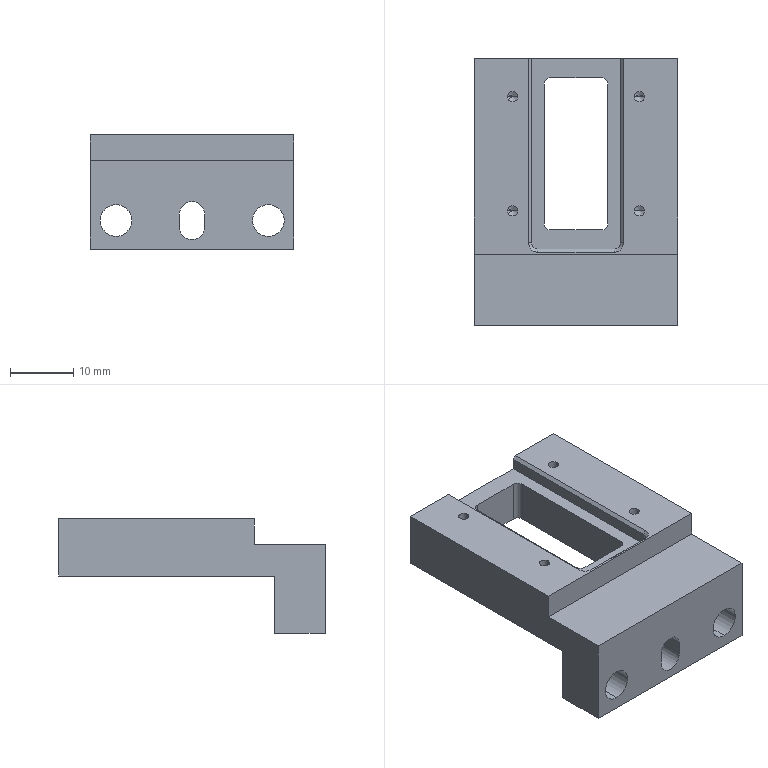NC program | NX | posted with a generic post | part box 32 x 42 x 18 mm
Whole program:
N10 G17 G21 G94 G90
(FLOOR_WALL_1_COPY_1 , TOOL : D6)
N12 T06 M6
N14 G54
N16 G17 G0 G90 X25. Y3.636 B0. C0. S9500 M3
N18 G43 Z30. H6
N20 Z0.506
N22 G94 G1 Z-0.494 F1000.
N24 X21.214 Y0.46
N26 G3 X21. Y0. R0.6
N28 G1 Y-16. F2500.
N30 X-9.9
N32 Y16.
N34 X21.
N36 Y0.
N38 X16.8
N40 Y-11.8
N42 X-5.7
N44 Y11.8
N46 X16.8
N48 Y0.
N50 X12.6
N52 Y-7.6
N54 X-1.5
N56 Y7.6
N58 X12.6
N60 Y0.
N62 X8.4
N64 Y-3.4
N66 X2.7
N68 Y3.4
N70 X8.4
N72 Y0.
N74 X5.7
N76 Y-0.7
N78 X5.4
N80 Y0.7
N82 X5.7
N84 Y0.
N86 G3 X5.914 Y-0.46 R0.6
N88 G1 Z0.506
N90 G0 X25. Y3.636 Z0.011
N92 G1 Z-0.989 F1000.
N94 X21.214 Y0.46
N96 G3 X21. Y0. R0.6
N98 G1 Y-16. F2500.
N100 X-9.9
N102 Y16.
N104 X21.
N106 Y0.
N108 X16.8
N110 Y-11.8
N112 X-5.7
N114 Y11.8
N116 X16.8
N118 Y0.
N120 X12.6
N122 Y-7.6
N124 X-1.5
N126 Y7.6
N128 X12.6
N130 Y0.
N132 X8.4
N134 Y-3.4
N136 X2.7
N138 Y3.4
N140 X8.4
N142 Y0.
N144 X5.7
N146 Y-0.7
N148 X5.4
N150 Y0.7
N152 X5.7
N154 Y0.
N156 G3 X5.914 Y-0.46 R0.6
N158 G1 Z0.011
N160 G0 X25. Y3.636 Z-0.483
N162 G1 Z-1.483 F1000.
N164 X21.214 Y0.46
N166 G3 X21. Y0. R0.6
N168 G1 Y-16. F2500.
N170 X-9.9
N172 Y16.
N174 X21.
N176 Y0.
N178 X16.8
N180 Y-11.8
N182 X-5.7
N184 Y11.8
N186 X16.8
N188 Y0.
N190 X12.6
N192 Y-7.6
N194 X-1.5
N196 Y7.6
N198 X12.6
N200 Y0.
N202 X8.4
N204 Y-3.4
N206 X2.7
N208 Y3.4
N210 X8.4
N212 Y0.
N214 X5.7
N216 Y-0.7
N218 X5.4
N220 Y0.7
N222 X5.7
N224 Y0.
N226 G3 X5.914 Y-0.46 R0.6
N228 G1 Z-0.483
N230 G0 X25. Y3.636 Z-0.978
N232 G1 Z-1.978 F1000.
N234 X21.214 Y0.46
N236 G3 X21. Y0. R0.6
N238 G1 Y-16. F2500.
N240 X-9.9
N242 Y16.
N244 X21.
N246 Y0.
N248 X16.8
N250 Y-11.8
N252 X-5.7
N254 Y11.8
N256 X16.8
N258 Y0.
N260 X12.6
N262 Y-7.6
N264 X-1.5
N266 Y7.6
N268 X12.6
N270 Y0.
N272 X8.4
N274 Y-3.4
N276 X2.7
N278 Y3.4
N280 X8.4
N282 Y0.
N284 X5.7
N286 Y-0.7
N288 X5.4
N290 Y0.7
N292 X5.7
N294 Y0.
N296 G3 X5.914 Y-0.46 R0.6
N298 G1 Z-0.978
N300 G0 X25. Y3.636 Z-1.472
N302 G1 Z-2.472 F1000.
N304 X21.214 Y0.46
N306 G3 X21. Y0. R0.6
N308 G1 Y-16. F2500.
N310 X-9.9
N312 Y16.
N314 X21.
N316 Y0.
N318 X16.8
N320 Y-11.8
N322 X-5.7
N324 Y11.8
N326 X16.8
N328 Y0.
N330 X12.6
N332 Y-7.6
N334 X-1.5
N336 Y7.6
N338 X12.6
N340 Y0.
N342 X8.4
N344 Y-3.4
N346 X2.7
N348 Y3.4
N350 X8.4
N352 Y0.
N354 X5.7
N356 Y-0.7
N358 X5.4
N360 Y0.7
N362 X5.7
N364 Y0.
N366 G3 X5.914 Y-0.46 R0.6
N368 G1 Z-1.472
N370 G0 X25. Y3.636 Z-1.967
N372 G1 Z-2.967 F1000.
N374 X21.214 Y0.46
N376 G3 X21. Y0. R0.6
N378 G1 Y-16. F2500.
N380 X-9.9
N382 Y16.
N384 X21.
N386 Y0.
N388 X16.8
N390 Y-11.8
N392 X-5.7
N394 Y11.8
N396 X16.8
N398 Y0.
N400 X12.6
N402 Y-7.6
N404 X-1.5
N406 Y7.6
N408 X12.6
N410 Y0.
N412 X8.4
N414 Y-3.4
N416 X2.7
N418 Y3.4
N420 X8.4
N422 Y0.
N424 X5.7
N426 Y-0.7
N428 X5.4
N430 Y0.7
N432 X5.7
N434 Y0.
N436 G3 X5.914 Y-0.46 R0.6
N438 G1 Z-1.967
N440 G0 X25. Y3.636 Z-2.461
N442 G1 Z-3.461 F1000.
N444 X21.214 Y0.46
N446 G3 X21. Y0. R0.6
N448 G1 Y-16. F2500.
N450 X-9.9
N452 Y16.
N454 X21.
N456 Y0.
N458 X16.8
N460 Y-11.8
N462 X-5.7
N464 Y11.8
N466 X16.8
N468 Y0.
N470 X12.6
N472 Y-7.6
N474 X-1.5
N476 Y7.6
N478 X12.6
N480 Y0.
N482 X8.4
N484 Y-3.4
N486 X2.7
N488 Y3.4
N490 X8.4
N492 Y0.
N494 X5.7
N496 Y-0.7
N498 X5.4
N500 Y0.7
N502 X5.7
N504 Y0.
N506 G3 X5.914 Y-0.46 R0.6
N508 G1 Z-2.461
N510 G0 X25. Y3.636 Z-2.956
N512 G1 Z-3.956 F1000.
N514 X21.214 Y0.46
N516 G3 X21. Y0. R0.6
N518 G1 Y-16. F2500.
N520 X-9.9
N522 Y16.
N524 X21.
N526 Y0.
N528 X16.8
N530 Y-11.8
N532 X-5.7
N534 Y11.8
N536 X16.8
N538 Y0.
N540 X12.6
N542 Y-7.6
N544 X-1.5
N546 Y7.6
N548 X12.6
N550 Y0.
N552 X8.4
N554 Y-3.4
N556 X2.7
N558 Y3.4
N560 X8.4
N562 Y0.
N564 X5.7
N566 Y-0.7
N568 X5.4
N570 Y0.7
N572 X5.7
N574 Y0.
N576 G3 X5.914 Y-0.46 R0.6
N578 G1 Z-2.956
N580 G0 X25. Y3.636 Z-3.45
N582 G1 Z-4.45 F1000.
N584 X21.214 Y0.46
N586 G3 X21. Y0. R0.6
N588 G1 Y-16. F2500.
N590 X-9.9
N592 Y16.
N594 X21.
N596 Y0.
N598 X16.8
N600 Y-11.8
N602 X-5.7
N604 Y11.8
N606 X16.8
N608 Y0.
N610 X12.6
N612 Y-7.6
N614 X-1.5
N616 Y7.6
N618 X12.6
N620 Y0.
N622 X8.4
N624 Y-3.4
N626 X2.7
N628 Y3.4
N630 X8.4
N632 Y0.
N634 X5.7
N636 Y-0.7
N638 X5.4
N640 Y0.7
N642 X5.7
N644 Y0.
N646 G3 X5.914 Y-0.46 R0.6
N648 G1 Z-3.45
N650 G0 X25. Y3.636 Z-3.944
N652 G1 Z-4.944 F1000.
N654 X21.214 Y0.46
N656 G3 X21. Y0. R0.6
N658 G1 Y-16. F2500.
N660 X-9.9
N662 Y16.
N664 X21.
N666 Y0.
N668 X16.8
N670 Y-11.8
N672 X-5.7
N674 Y11.8
N676 X16.8
N678 Y0.
N680 X12.6
N682 Y-7.6
N684 X-1.5
N686 Y7.6
N688 X12.6
N690 Y0.
N692 X8.4
N694 Y-3.4
N696 X2.7
N698 Y3.4
N700 X8.4
N702 Y0.
N704 X5.7
N706 Y-0.7
N708 X5.4
N710 Y0.7
N712 X5.7
N714 Y0.
N716 G3 X5.914 Y-0.46 R0.6
N718 G1 Z-3.944
N720 G0 X25. Y3.636 Z-4.439
N722 G1 Z-5.439 F1000.
N724 X21.214 Y0.46
N726 G3 X21. Y0. R0.6
N728 G1 Y-16. F2500.
N730 X-9.9
N732 Y16.
N734 X21.
N736 Y0.
N738 X16.8
N740 Y-11.8
N742 X-5.7
N744 Y11.8
N746 X16.8
N748 Y0.
N750 X12.6
N752 Y-7.6
N754 X-1.5
N756 Y7.6
N758 X12.6
N760 Y0.
N762 X8.4
N764 Y-3.4
N766 X2.7
N768 Y3.4
N770 X8.4
N772 Y0.
N774 X5.7
N776 Y-0.7
N778 X5.4
N780 Y0.7
N782 X5.7
N784 Y0.
N786 G3 X5.914 Y-0.46 R0.6
N788 G1 Z-4.439
N790 G0 X25. Y3.636 Z-4.933
N792 G1 Z-5.933 F1000.
N794 X21.214 Y0.46
N796 G3 X21. Y0. R0.6
N798 G1 Y-16. F2500.
N800 X-9.9
N802 Y16.
N804 X21.
N806 Y0.
N808 X16.8
N810 Y-11.8
N812 X-5.7
N814 Y11.8
N816 X16.8
N818 Y0.
N820 X12.6
N822 Y-7.6
N824 X-1.5
N826 Y7.6
N828 X12.6
N830 Y0.
N832 X8.4
N834 Y-3.4
N836 X2.7
N838 Y3.4
N840 X8.4
N842 Y0.
N844 X5.7
N846 Y-0.7
N848 X5.4
N850 Y0.7
N852 X5.7
N854 Y0.
N856 G3 X5.914 Y-0.46 R0.6
N858 G1 Z-4.933
N860 G0 X25. Y3.636 Z-5.428
N862 G1 Z-6.428 F1000.
N864 X21.214 Y0.46
N866 G3 X21. Y0. R0.6
N868 G1 Y-16. F2500.
N870 X-9.9
N872 Y16.
N874 X21.
N876 Y0.
N878 X16.8
N880 Y-11.8
N882 X-5.7
N884 Y11.8
N886 X16.8
N888 Y0.
N890 X12.6
N892 Y-7.6
N894 X-1.5
N896 Y7.6
N898 X12.6
N900 Y0.
N902 X8.4
N904 Y-3.4
N906 X2.7
N908 Y3.4
N910 X8.4
N912 Y0.
N914 X5.7
N916 Y-0.7
N918 X5.4
N920 Y0.7
N922 X5.7
N924 Y0.
N926 G3 X5.914 Y-0.46 R0.6
N928 G1 Z-5.428
N930 G0 X25. Y3.636 Z-5.922
N932 G1 Z-6.922 F1000.
N934 X21.214 Y0.46
N936 G3 X21. Y0. R0.6
N938 G1 Y-16. F2500.
N940 X-9.9
N942 Y16.
N944 X21.
N946 Y0.
N948 X16.8
N950 Y-11.8
N952 X-5.7
N954 Y11.8
N956 X16.8
N958 Y0.
N960 X12.6
N962 Y-7.6
N964 X-1.5
N966 Y7.6
N968 X12.6
N970 Y0.
N972 X8.4
N974 Y-3.4
N976 X2.7
N978 Y3.4
N980 X8.4
N982 Y0.
N984 X5.7
N986 Y-0.7
N988 X5.4
N990 Y0.7
N992 X5.7
N994 Y0.
N996 G3 X5.914 Y-0.46 R0.6
N998 G1 Z-5.922
N1000 G0 X25. Y3.636 Z-6.417
N1002 G1 Z-7.417 F1000.
N1004 X21.214 Y0.46
N1006 G3 X21. Y0. R0.6
N1008 G1 Y-16. F2500.
N1010 X-9.9
N1012 Y16.
N1014 X21.
N1016 Y0.
N1018 X16.8
N1020 Y-11.8
N1022 X-5.7
N1024 Y11.8
N1026 X16.8
N1028 Y0.
N1030 X12.6
N1032 Y-7.6
N1034 X-1.5
N1036 Y7.6
N1038 X12.6
N1040 Y0.
N1042 X8.4
N1044 Y-3.4
N1046 X2.7
N1048 Y3.4
N1050 X8.4
N1052 Y0.
N1054 X5.7
N1056 Y-0.7
N1058 X5.4
N1060 Y0.7
N1062 X5.7
N1064 Y0.
N1066 G3 X5.914 Y-0.46 R0.6
N1068 G1 Z-6.417
N1070 G0 X25. Y3.636 Z-6.911
N1072 G1 Z-7.911 F1000.
N1074 X21.214 Y0.46
N1076 G3 X21. Y0. R0.6
N1078 G1 Y-16. F2500.
N1080 X-9.9
N1082 Y16.
N1084 X21.
N1086 Y0.
N1088 X16.8
N1090 Y-11.8
N1092 X-5.7
N1094 Y11.8
N1096 X16.8
N1098 Y0.
N1100 X12.6
N1102 Y-7.6
N1104 X-1.5
N1106 Y7.6
N1108 X12.6
N1110 Y0.
N1112 X8.4
N1114 Y-3.4
N1116 X2.7
N1118 Y3.4
N1120 X8.4
N1122 Y0.
N1124 X5.7
N1126 Y-0.7
N1128 X5.4
N1130 Y0.7
N1132 X5.7
N1134 Y0.
N1136 G3 X5.914 Y-0.46 R0.6
N1138 G1 Z-6.911
N1140 G0 X25. Y3.636 Z-7.406
N1142 G1 Z-8.406 F1000.
N1144 X21.214 Y0.46
N1146 G3 X21. Y0. R0.6
N1148 G1 Y-16. F2500.
N1150 X-9.9
N1152 Y16.
N1154 X21.
N1156 Y0.
N1158 X16.8
N1160 Y-11.8
N1162 X-5.7
N1164 Y11.8
N1166 X16.8
N1168 Y0.
N1170 X12.6
N1172 Y-7.6
N1174 X-1.5
N1176 Y7.6
N1178 X12.6
N1180 Y0.
N1182 X8.4
N1184 Y-3.4
N1186 X2.7
N1188 Y3.4
N1190 X8.4
N1192 Y0.
N1194 X5.7
N1196 Y-0.7
N1198 X5.4
N1200 Y0.7
N1202 X5.7
N1204 Y0.
N1206 G3 X5.914 Y-0.46 R0.6
N1208 G1 Z-7.406
N1210 G0 X25. Y3.636 Z-7.9
N1212 G1 Z-8.9 F1000.
N1214 X21.214 Y0.46
N1216 G3 X21. Y0. R0.6
N1218 G1 Y-16. F2500.
N1220 X-9.9
N1222 Y16.
N1224 X21.
N1226 Y0.
N1228 X16.8
N1230 Y-11.8
N1232 X-5.7
N1234 Y11.8
N1236 X16.8
N1238 Y0.
N1240 X12.6
N1242 Y-7.6
N1244 X-1.5
N1246 Y7.6
N1248 X12.6
N1250 Y0.
N1252 X8.4
N1254 Y-3.4
N1256 X2.7
N1258 Y3.4
N1260 X8.4
N1262 Y0.
N1264 X5.7
N1266 Y-0.7
N1268 X5.4
N1270 Y0.7
N1272 X5.7
N1274 Y0.
N1276 G3 X5.914 Y-0.46 R0.6
N1278 G1 Z-7.9
N1280 G0 Z30.
(FLOOR_WALL_1_1_COPY_1 , TOOL : D6)
N1282 X25.123 Y19.995
N1284 Z-7.5
N1286 G1 Z-9. F1250.
N1288 X24.3 Y19.52
N1290 G3 X24. Y19. R0.6
N1292 G1 Y-19.
N1294 X21.192
N1296 Y19.
N1298 X18.383
N1300 Y-19.
N1302 X15.575
N1304 Y19.
N1306 X12.767
N1308 Y-19.
N1310 X9.958
N1312 Y19.
N1314 X7.15
N1316 Y-19.
N1318 X4.342
N1320 Y19.
N1322 X1.533
N1324 Y-19.
N1326 X-1.275
N1328 Y19.
N1330 X-4.083
N1332 Y-19.
N1334 X-6.892
N1336 Y19.
N1338 X-9.7
N1340 Y-19.
N1342 G3 X-9.4 Y-19.52 R0.6
N1344 G1 X-7.702 Y-20.5
N1346 Z-7.5
N1348 G0 Z1.1
N1350 X-8.002 Y20.5
N1352 Z-7.5
N1354 G1 Z-9.
N1356 X-9.7 Y19.52
N1358 G3 X-10. Y19. R0.6
N1360 G1 Y-19.
N1362 G3 X-9.7 Y-19.52 R0.6
N1364 G1 X-8.002 Y-20.5
N1366 Z-7.5
N1368 G0 Z30.
N1370 M5
(PLANAR_MILL_COPY_COPY_2 , TOOL : D6A45)
N1372 T07 M6
N1374 G54
N1376 G17 G0 G90 X-11. Y1.27 B0. C0. S9500 M3
N1378 G43 Z30. H7
N1380 Z0.5
N1382 G94 G1 Z-1. F1250.
N1384 X-11.7 Y0.866
N1386 G3 X-12.2 Y0. R1.
N1388 G1 Y-15.8
N1390 G2 X-13.2 Y-16.8 R1.
N1392 G1 X-20.8
N1394 G2 X-21.8 Y-15.8 R1.
N1396 G1 Y15.8
N1398 G2 X-20.8 Y16.8 R1.
N1400 G1 X-13.2
N1402 G2 X-12.2 Y15.8 R1.
N1404 G1 Y0.
N1406 G3 X-11.7 Y-0.866 R1.
N1408 G1 X-11. Y-1.27
N1410 Z0.5
N1412 G0 Z30.
N1414 M5
N1416 M2